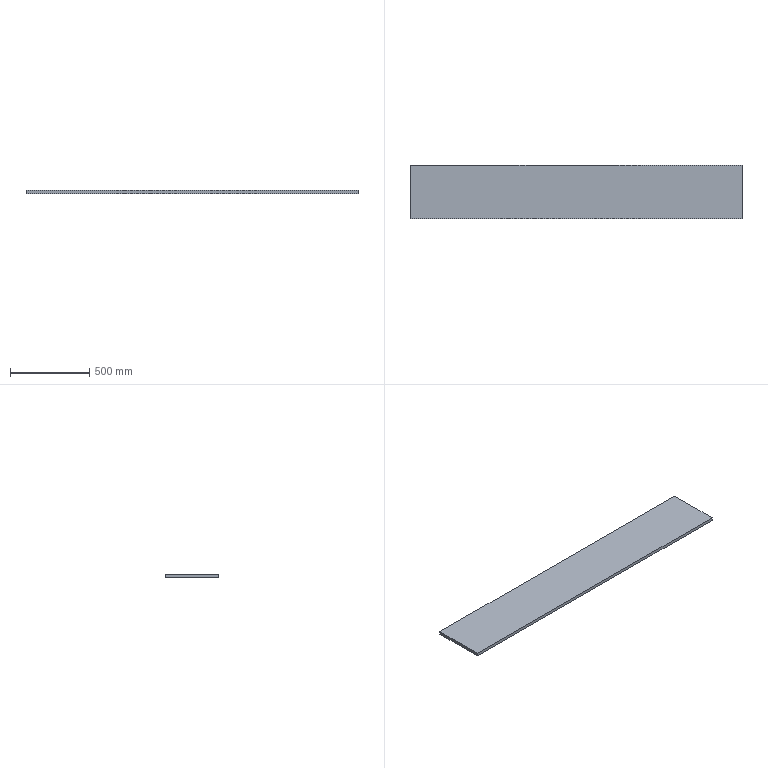Part | SolidWorks | features Extrusion 1 | 1 solid | 6 faces | box 2100 x 336 x 20 mm | volume 14112000 mm3 | plane 6
STEP:
#1=CARTESIAN_POINT('',(-1050.,168.,-10.));
#2=VERTEX_POINT('',#1);
#3=CARTESIAN_POINT('',(-1050.,-168.,-10.));
#4=VERTEX_POINT('',#3);
#5=CARTESIAN_POINT('',(-1050.,168.,-10.));
#6=DIRECTION('',(0.,-1.,0.));
#7=VECTOR('',#6,1000.);
#8=LINE('',#5,#7);
#9=EDGE_CURVE('',#2,#4,#8,.T.);
#10=ORIENTED_EDGE('',*,*,#9,.T.);
#11=CARTESIAN_POINT('',(-1050.,-168.,10.));
#12=VERTEX_POINT('',#11);
#13=CARTESIAN_POINT('',(-1050.,-168.,10.));
#14=DIRECTION('',(0.,0.,-1.));
#15=VECTOR('',#14,1000.);
#16=LINE('',#13,#15);
#17=EDGE_CURVE('',#12,#4,#16,.T.);
#18=ORIENTED_EDGE('',*,*,#17,.F.);
#19=CARTESIAN_POINT('',(-1050.,168.,10.));
#20=VERTEX_POINT('',#19);
#21=CARTESIAN_POINT('',(-1050.,168.,10.));
#22=DIRECTION('',(0.,-1.,0.));
#23=VECTOR('',#22,1000.);
#24=LINE('',#21,#23);
#25=EDGE_CURVE('',#20,#12,#24,.T.);
#26=ORIENTED_EDGE('',*,*,#25,.F.);
#27=CARTESIAN_POINT('',(-1050.,168.,10.));
#28=DIRECTION('',(0.,0.,-1.));
#29=VECTOR('',#28,1000.);
#30=LINE('',#27,#29);
#31=EDGE_CURVE('',#20,#2,#30,.T.);
#32=ORIENTED_EDGE('',*,*,#31,.T.);
#33=EDGE_LOOP('',(#10,#18,#26,#32));
#34=FACE_OUTER_BOUND('',#33,.T.);
#35=CARTESIAN_POINT('',(-1050.,168.,10.));
#36=DIRECTION('',(1.,0.,0.));
#37=DIRECTION('',(0.,1.,0.));
#38=AXIS2_PLACEMENT_3D('',#35,#36,#37);
#39=PLANE('',#38);
#40=ADVANCED_FACE('',(#34),#39,.F.);
#41=CARTESIAN_POINT('',(1050.,-168.,-10.));
#42=VERTEX_POINT('',#41);
#43=CARTESIAN_POINT('',(-1050.,-168.,-10.));
#44=DIRECTION('',(1.,0.,0.));
#45=VECTOR('',#44,1000.);
#46=LINE('',#43,#45);
#47=EDGE_CURVE('',#4,#42,#46,.T.);
#48=ORIENTED_EDGE('',*,*,#47,.T.);
#49=CARTESIAN_POINT('',(1050.,-168.,10.));
#50=VERTEX_POINT('',#49);
#51=CARTESIAN_POINT('',(1050.,-168.,10.));
#52=DIRECTION('',(0.,0.,-1.));
#53=VECTOR('',#52,1000.);
#54=LINE('',#51,#53);
#55=EDGE_CURVE('',#50,#42,#54,.T.);
#56=ORIENTED_EDGE('',*,*,#55,.F.);
#57=CARTESIAN_POINT('',(-1050.,-168.,10.));
#58=DIRECTION('',(1.,0.,0.));
#59=VECTOR('',#58,1000.);
#60=LINE('',#57,#59);
#61=EDGE_CURVE('',#12,#50,#60,.T.);
#62=ORIENTED_EDGE('',*,*,#61,.F.);
#63=ORIENTED_EDGE('',*,*,#17,.T.);
#64=EDGE_LOOP('',(#48,#56,#62,#63));
#65=FACE_OUTER_BOUND('',#64,.T.);
#66=CARTESIAN_POINT('',(-1050.,-168.,10.));
#67=DIRECTION('',(0.,1.,0.));
#68=DIRECTION('',(0.,0.,1.));
#69=AXIS2_PLACEMENT_3D('',#66,#67,#68);
#70=PLANE('',#69);
#71=ADVANCED_FACE('',(#65),#70,.F.);
#72=CARTESIAN_POINT('',(1050.,168.,-10.));
#73=VERTEX_POINT('',#72);
#74=CARTESIAN_POINT('',(1050.,168.,-10.));
#75=DIRECTION('',(0.,1.,0.));
#76=VECTOR('',#75,1000.);
#77=LINE('',#74,#76);
#78=EDGE_CURVE('',#42,#73,#77,.T.);
#79=ORIENTED_EDGE('',*,*,#78,.T.);
#80=CARTESIAN_POINT('',(1050.,168.,10.));
#81=VERTEX_POINT('',#80);
#82=CARTESIAN_POINT('',(1050.,168.,10.));
#83=DIRECTION('',(0.,0.,-1.));
#84=VECTOR('',#83,1000.);
#85=LINE('',#82,#84);
#86=EDGE_CURVE('',#81,#73,#85,.T.);
#87=ORIENTED_EDGE('',*,*,#86,.F.);
#88=CARTESIAN_POINT('',(1050.,168.,10.));
#89=DIRECTION('',(0.,1.,0.));
#90=VECTOR('',#89,1000.);
#91=LINE('',#88,#90);
#92=EDGE_CURVE('',#50,#81,#91,.T.);
#93=ORIENTED_EDGE('',*,*,#92,.F.);
#94=ORIENTED_EDGE('',*,*,#55,.T.);
#95=EDGE_LOOP('',(#79,#87,#93,#94));
#96=FACE_OUTER_BOUND('',#95,.T.);
#97=CARTESIAN_POINT('',(1050.,168.,10.));
#98=DIRECTION('',(-1.,0.,0.));
#99=DIRECTION('',(0.,0.,1.));
#100=AXIS2_PLACEMENT_3D('',#97,#98,#99);
#101=PLANE('',#100);
#102=ADVANCED_FACE('',(#96),#101,.F.);
#103=CARTESIAN_POINT('',(-1050.,168.,-10.));
#104=DIRECTION('',(-1.,0.,0.));
#105=VECTOR('',#104,1000.);
#106=LINE('',#103,#105);
#107=EDGE_CURVE('',#73,#2,#106,.T.);
#108=ORIENTED_EDGE('',*,*,#107,.T.);
#109=ORIENTED_EDGE('',*,*,#31,.F.);
#110=CARTESIAN_POINT('',(-1050.,168.,10.));
#111=DIRECTION('',(-1.,0.,0.));
#112=VECTOR('',#111,1000.);
#113=LINE('',#110,#112);
#114=EDGE_CURVE('',#81,#20,#113,.T.);
#115=ORIENTED_EDGE('',*,*,#114,.F.);
#116=ORIENTED_EDGE('',*,*,#86,.T.);
#117=EDGE_LOOP('',(#108,#109,#115,#116));
#118=FACE_OUTER_BOUND('',#117,.T.);
#119=CARTESIAN_POINT('',(-1050.,168.,10.));
#120=DIRECTION('',(0.,-1.,0.));
#121=DIRECTION('',(0.,0.,-1.));
#122=AXIS2_PLACEMENT_3D('',#119,#120,#121);
#123=PLANE('',#122);
#124=ADVANCED_FACE('',(#118),#123,.F.);
#125=ORIENTED_EDGE('',*,*,#25,.T.);
#126=ORIENTED_EDGE('',*,*,#61,.T.);
#127=ORIENTED_EDGE('',*,*,#92,.T.);
#128=ORIENTED_EDGE('',*,*,#114,.T.);
#129=EDGE_LOOP('',(#125,#126,#127,#128));
#130=FACE_OUTER_BOUND('',#129,.T.);
#131=CARTESIAN_POINT('',(-1050.,-168.,10.));
#132=DIRECTION('',(0.,0.,1.));
#133=DIRECTION('',(1.,0.,0.));
#134=AXIS2_PLACEMENT_3D('',#131,#132,#133);
#135=PLANE('',#134);
#136=ADVANCED_FACE('',(#130),#135,.T.);
#137=ORIENTED_EDGE('',*,*,#9,.F.);
#138=ORIENTED_EDGE('',*,*,#107,.F.);
#139=ORIENTED_EDGE('',*,*,#78,.F.);
#140=ORIENTED_EDGE('',*,*,#47,.F.);
#141=EDGE_LOOP('',(#137,#138,#139,#140));
#142=FACE_OUTER_BOUND('',#141,.T.);
#143=CARTESIAN_POINT('',(-1050.,-168.,-10.));
#144=DIRECTION('',(0.,0.,1.));
#145=DIRECTION('',(1.,0.,0.));
#146=AXIS2_PLACEMENT_3D('',#143,#144,#145);
#147=PLANE('',#146);
#148=ADVANCED_FACE('',(#142),#147,.F.);
#149=CLOSED_SHELL('',(#40,#71,#102,#124,#136,#148));
#150=MANIFOLD_SOLID_BREP('',#149);
#151=CARTESIAN_POINT('',(0.,0.,0.));
#152=DIRECTION('',(0.,0.,1.));
#153=DIRECTION('',(1.,0.,0.));
#154=AXIS2_PLACEMENT_3D('',#151,#152,#153);
#155=(LENGTH_UNIT()NAMED_UNIT(*)SI_UNIT(.MILLI.,.METRE.));
#156=UNCERTAINTY_MEASURE_WITH_UNIT(LENGTH_MEASURE(0.00001),#155,'','');
#157=(NAMED_UNIT(*)PLANE_ANGLE_UNIT()SI_UNIT($,.RADIAN.));
#158=(NAMED_UNIT(*)SI_UNIT($,.STERADIAN.)SOLID_ANGLE_UNIT());
#159=(GEOMETRIC_REPRESENTATION_CONTEXT(3)GLOBAL_UNCERTAINTY_ASSIGNED_CONTEXT((#156))GLOBAL_UNIT_ASSIGNED_CONTEXT((#155,#157,#158))REPRESENTATION_CONTEXT('',''));
#160=ADVANCED_BREP_SHAPE_REPRESENTATION('',(#150,#154),#159);